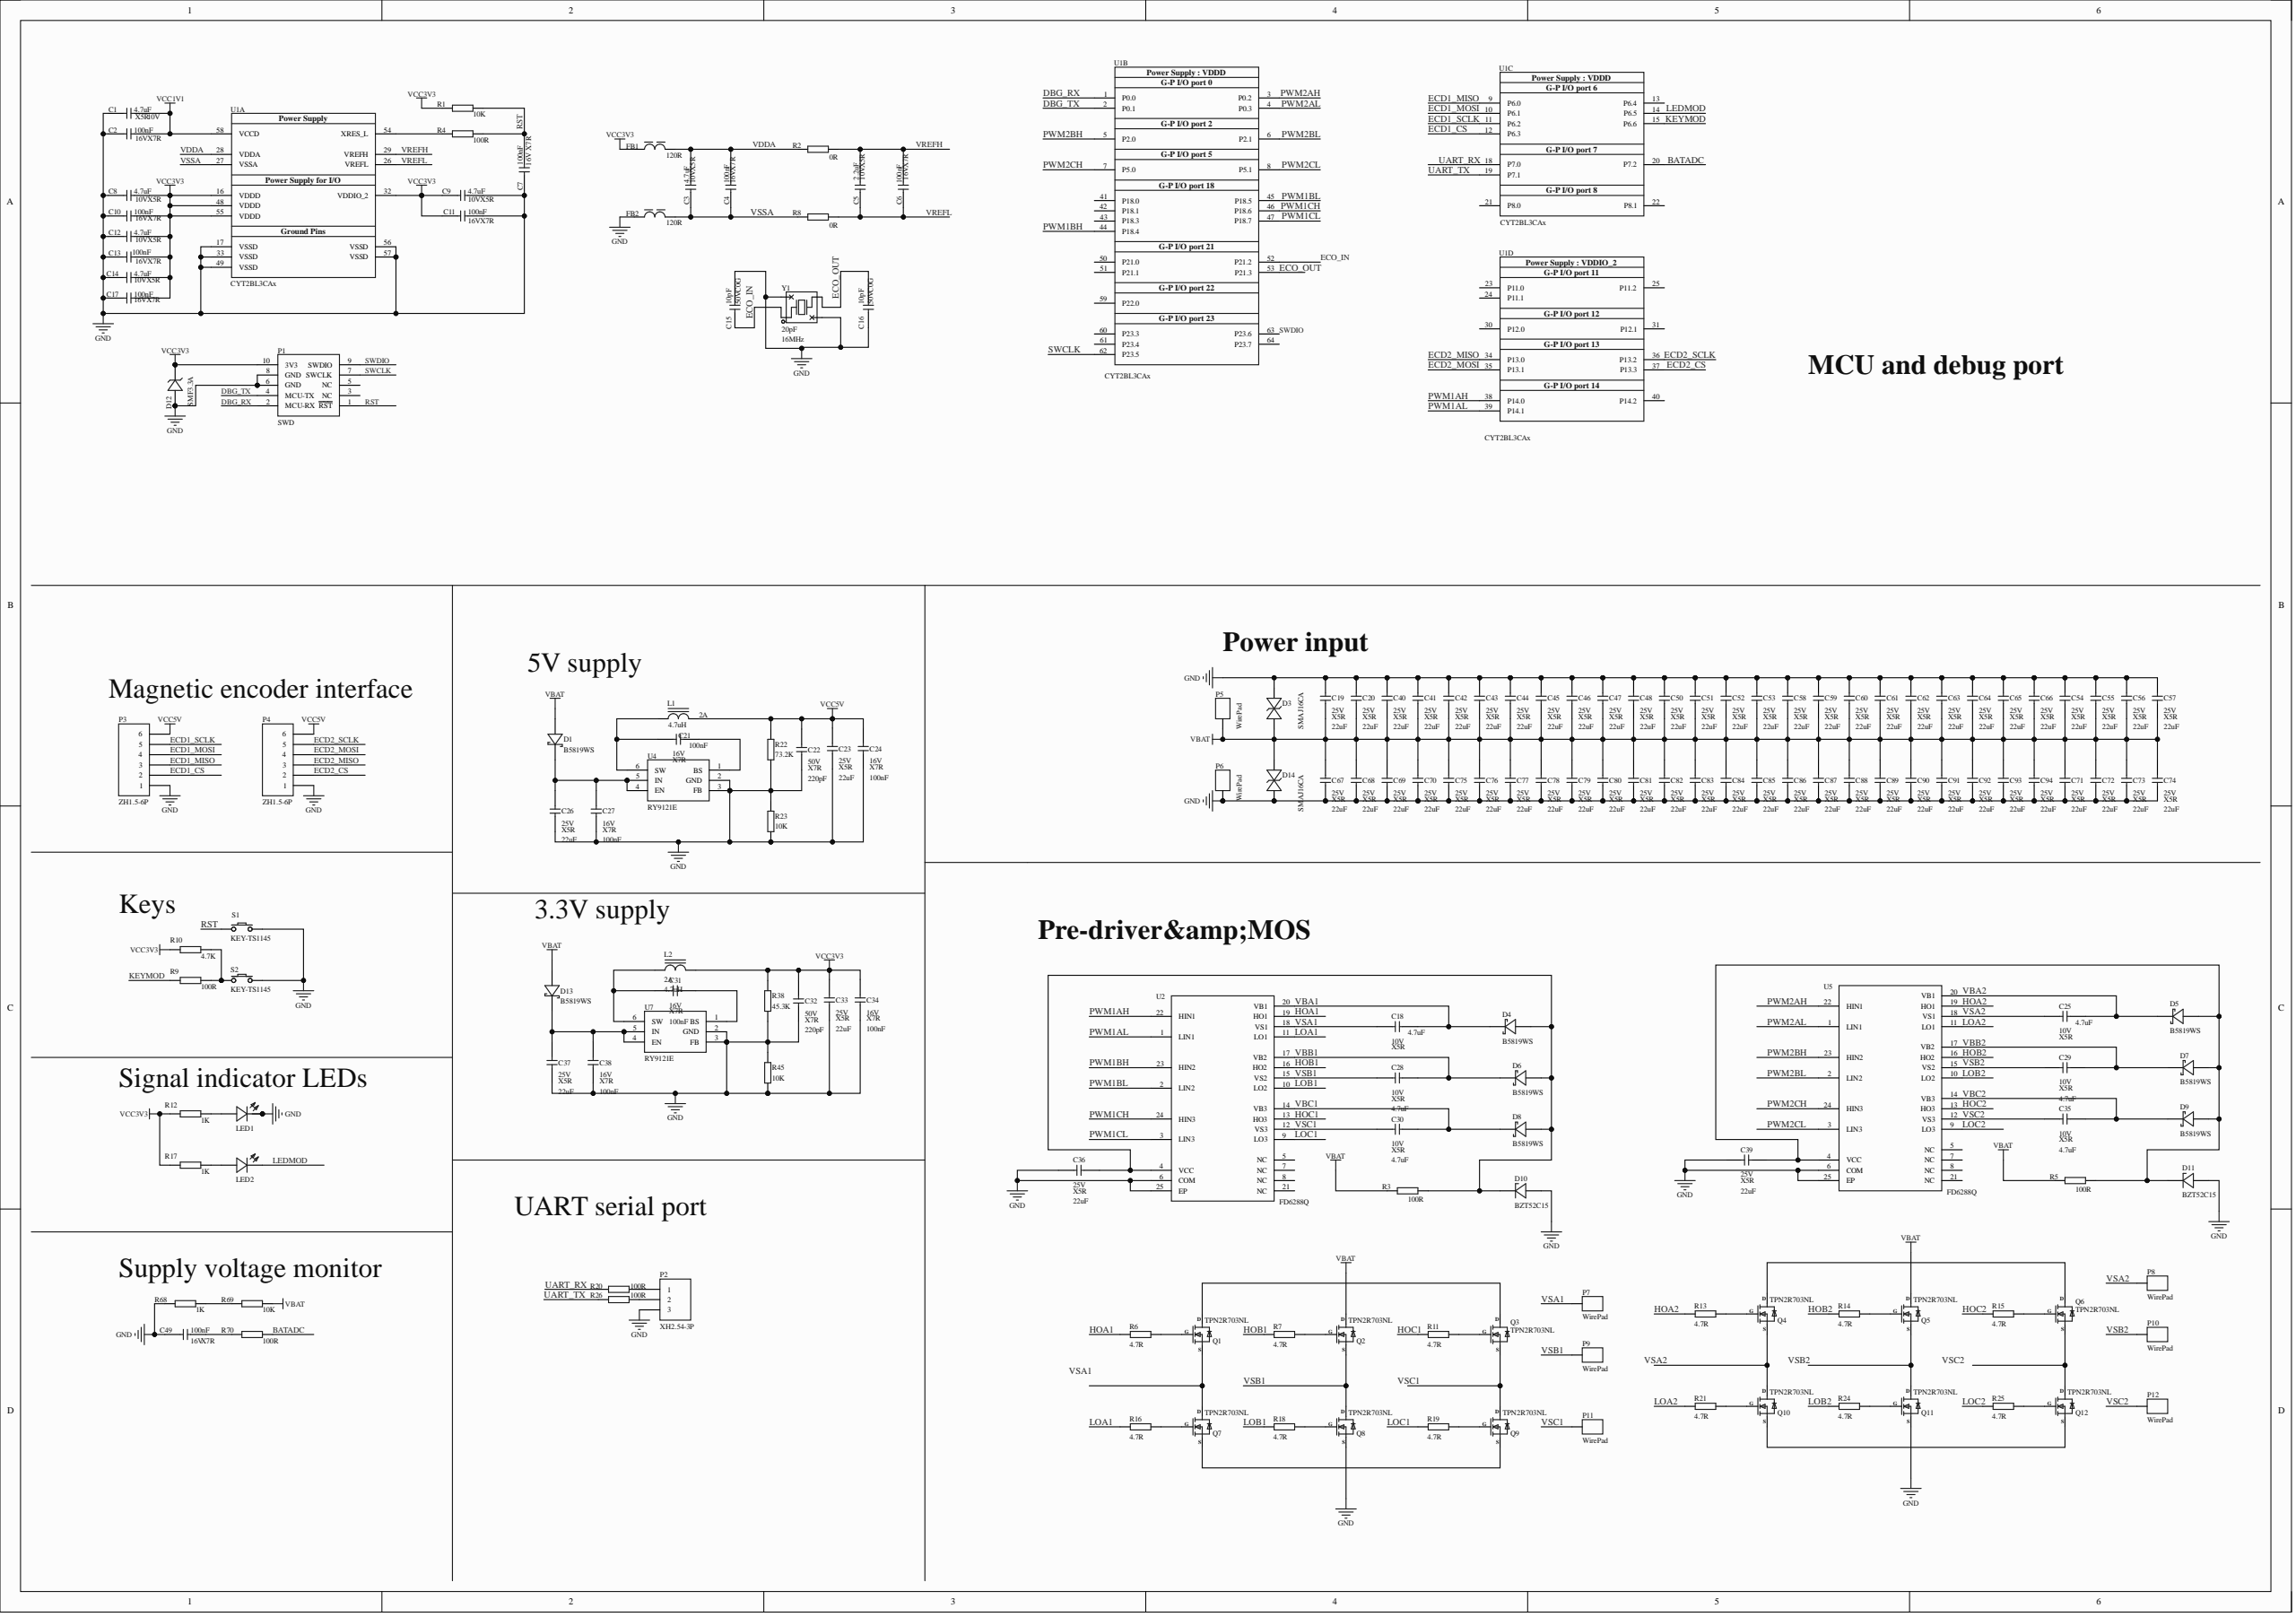Circuit board | Altium Designer | 176 parts | 102 nets
Bill of materials:
Comment,Description,Designator,Footprint,LibRef,Quantity
"","SMD ceramic capacitor; MLCC; 0402(1005);","C1, C2, C3, C4, C5, C6, C7, C8, C9, C10, C11, C12, C13, C14, C15, C16, C17, C18, C21, C22, C24, C25, C27, C28, C29, C30, C31, C32, C34, C35, C38, C49","CAPC1005[0402]S-N","=Value +' '+ Voltage + ' ' + Type","32"
"","SMD ceramic capacitor; MLCC; 0805(2012);","C19, C20, C23, C26, C33, C36, C37, C39, C40, C41, C42, C43, C44, C45, C46, C47, C48, C50, C51, C52, C53, C54, C55, C56, C57, C58, C59, C60, C61, C62, C63, C64, C65, C66, C67, C68, C69, C70, C71, C72, C73, C74, C75, C76, C77, C78, C79, C80, C81, C82, C83, C84, C85, C86, C87, C88, C89, C90, C91, C92, C93, C94","CAPC2012[0805]S-N","=Value +' '+ Voltage + ' ' + Type","62"
"B5819WS","B5819WS Schottky diode","D1, D4, D5, D6, D7, D8, D9, D13","SOD-323","B5819WS","8"
"SMAJ16CA","TRANSIENT VOLTAGE  SUPPRESSOR DIODE","D3, D14","SMA[DO-214AC]-Bi","SMAJ16CA","2"
"BZT52C15","Zener diode (voltage regulator)","D10, D11","SOD-123-L","BZT52C15","2"
"SMF3.3A","TRANSIENT VOLTAGE  SUPPRESSOR DIODE","D12","SOD-123-FL","SMF3.3A","1"
"","SMD ferrite bead","FB1, FB2","INDC1005[0402]S","=Value + ' ' + Frequency +' '+ Imax","2"
"","Power inductor","L1, L2","SLO2520","=Value + ' ' + Imax","2"
"Red SMD LED","Red SMD LED","LED1","LEDC1608(0603)-L","红色贴片LED","1"
"Blue SMD LED","Blue SMD LED","LED2","LEDC1608(0603)-L","蓝色贴片LED","1"
"SWD Header 5x2","SWD debug interface 2x5pin dual-row pin header","P1","HDR2X5-OB","SWD Header 5x2","1"
"XH2.54-3P","XH2.54-3P","P2","XH2.54-3P-SH","XH2.54-3P","1"
"ZH1.5-6P","ZH1.5-6P","P3, P4","ZH1.5-6P-SH","ZH1.5-6P","2"
"WirePad","Cable wire pad","P5, P6, P7, P8, P9, P10, P11, P12","WirePad-4x6","WirePad","8"
"TPN2R703NL","Toshiba N-channel MOS","Q1, Q2, Q3, Q4, Q5, Q6, Q7, Q8, Q9, Q10, Q11, Q12","TSON3x3","TPN2R703NL","12"
"","SMD resistor","R1, R2, R3, R4, R5, R6, R7, R8, R9, R10, R11, R12, R13, R14, R15, R16, R17, R18, R19, R20, R21, R22, R23, R24, R25, R26, R38, R45, R68, R69, R70","RESC1005[0402]S-N","=Value+' '+Tolerance","31"
"KEY-TS1145","3x4x2.5 4-pin key SMD vertical press","S1, S2","TS1145-B-A","KEY-TS1145","2"
"CYT2BL3CAx","CYT2BL3CAx","U1","LQFP64_L","CYT2BL3CAx","1"
"FD6288Q","FD6288Q three-phase gate driver","U2, U5","QFN24-4x4-L","FD6288Q","2"
"RY9121E","17V 2A 1.2MHz Synchronous Step-Down Regulator","U4, U7","SOT-23-6","RY9121E","2"
"","Four-pin passive crystal oscillator Crystal Oscillator","Y1","X3225-4","=Frequency+' '+Load_Capactiance","1"
Netlist (Protel format):
[
C1
CAPC1005[0402]S-N




]
[
C2
CAPC1005[0402]S-N




]
[
C3
CAPC1005[0402]S-N




]
[
C4
CAPC1005[0402]S-N




]
[
C5
CAPC1005[0402]S-N




]
[
C6
CAPC1005[0402]S-N




]
[
C7
CAPC1005[0402]S-N




]
[
C8
CAPC1005[0402]S-N




]
[
C9
CAPC1005[0402]S-N




]
[
C10
CAPC1005[0402]S-N




]
[
C11
CAPC1005[0402]S-N




]
[
C12
CAPC1005[0402]S-N




]
[
C13
CAPC1005[0402]S-N




]
[
C14
CAPC1005[0402]S-N




]
[
C15
CAPC1005[0402]S-N




]
[
C16
CAPC1005[0402]S-N




]
[
C17
CAPC1005[0402]S-N




]
[
C18
CAPC1005[0402]S-N




]
[
C19
CAPC2012[0805]S-N




]
[
C20
CAPC2012[0805]S-N




]
[
C21
CAPC1005[0402]S-N




]
[
C22
CAPC1005[0402]S-N




]
[
C23
CAPC2012[0805]S-N




]
[
C24
CAPC1005[0402]S-N




]
[
C25
CAPC1005[0402]S-N




]
[
C26
CAPC2012[0805]S-N




]
[
C27
CAPC1005[0402]S-N




]
[
C28
CAPC1005[0402]S-N




]
[
C29
CAPC1005[0402]S-N




]
[
C30
CAPC1005[0402]S-N




]
[
C31
CAPC1005[0402]S-N




]
[
C32
CAPC1005[0402]S-N




]
[
C33
CAPC2012[0805]S-N




]
[
C34
CAPC1005[0402]S-N




]
[
C35
CAPC1005[0402]S-N




]
[
C36
CAPC2012[0805]S-N




]
[
C37
CAPC2012[0805]S-N




]
[
C38
CAPC1005[0402]S-N




]
[
C39
CAPC2012[0805]S-N




]
[
C40
CAPC2012[0805]S-N




]
[
C41
CAPC2012[0805]S-N




]
[
C42
CAPC2012[0805]S-N




]
[
C43
CAPC2012[0805]S-N




]
[
C44
CAPC2012[0805]S-N




]
[
C45
CAPC2012[0805]S-N




]
[
C46
CAPC2012[0805]S-N




]
[
C47
CAPC2012[0805]S-N




]
[
C48
CAPC2012[0805]S-N




]
[
C49
CAPC1005[0402]S-N




]
[
C50
CAPC2012[0805]S-N




]
[
C51
CAPC2012[0805]S-N




]
[
C52
CAPC2012[0805]S-N




]
[
C53
CAPC2012[0805]S-N




]
[
C54
CAPC2012[0805]S-N




]
[
C55
CAPC2012[0805]S-N




]
[
C56
CAPC2012[0805]S-N




]
[
C57
CAPC2012[0805]S-N




]
[
C58
CAPC2012[0805]S-N




]
[
C59
CAPC2012[0805]S-N




]
[
C60
CAPC2012[0805]S-N




]
[
C61
CAPC2012[0805]S-N




]
[
C62
CAPC2012[0805]S-N




]
[
C63
CAPC2012[0805]S-N




]
[
C64
CAPC2012[0805]S-N




]
[
C65
CAPC2012[0805]S-N




]
[
C66
CAPC2012[0805]S-N




]
[
C67
CAPC2012[0805]S-N




]
[
C68
CAPC2012[0805]S-N




]
[
C69
CAPC2012[0805]S-N




]
[
C70
CAPC2012[0805]S-N




]
[
C71
CAPC2012[0805]S-N




]
[
C72
CAPC2012[0805]S-N




]
[
C73
CAPC2012[0805]S-N




]
[
C74
CAPC2012[0805]S-N




]
[
C75
CAPC2012[0805]S-N




]
[
C76
CAPC2012[0805]S-N




]
[
C77
CAPC2012[0805]S-N




]
[
C78
CAPC2012[0805]S-N




]
[
C79
CAPC2012[0805]S-N




]
[
C80
CAPC2012[0805]S-N




]
[
C81
CAPC2012[0805]S-N




]
[
C82
CAPC2012[0805]S-N




]
[
C83
CAPC2012[0805]S-N




]
[
C84
CAPC2012[0805]S-N




]
[
C85
CAPC2012[0805]S-N




]
[
C86
CAPC2012[0805]S-N




]
[
C87
CAPC2012[0805]S-N




]
[
C88
CAPC2012[0805]S-N




]
[
C89
CAPC2012[0805]S-N




]
[
C90
CAPC2012[0805]S-N




]
[
C91
CAPC2012[0805]S-N




]
[
C92
CAPC2012[0805]S-N




]
[
C93
CAPC2012[0805]S-N




]
[
C94
CAPC2012[0805]S-N




]
[
D1
SOD-323
B5819WS



]
[
D3
SMA[DO-214AC]-Bi
SMAJ16CA



]
[
D4
SOD-323
B5819WS



]
[
D5
SOD-323
B5819WS



]
[
D6
SOD-323
B5819WS



]
[
D7
SOD-323
B5819WS



]
[
D8
SOD-323
B5819WS



]
[
D9
SOD-323
B5819WS



]
[
D10
SOD-123-L
BZT52C15



]
[
D11
SOD-123-L
BZT52C15



]
[
D12
SOD-123-FL
SMF3.3A



]
[
D13
SOD-323
B5819WS



]
[
D14
SMA[DO-214AC]-Bi
SMAJ16CA



]
[
FB1
INDC1005[0402]S




]
[
FB2
INDC1005[0402]S




]
[
L1
SLO2520




]
[
L2
SLO2520




]
[
LED1
LEDC1608(0603)-L
Red SMD LED



]
[
LED2
LEDC1608(0603)-L
Blue SMD LED



]
[
P1
HDR2X5-OB
SWD Header 5x2



]
[
P2
XH2.54-3P-SH
XH2.54-3P



]
[
P3
ZH1.5-6P-SH
ZH1.5-6P



]
[
P4
ZH1.5-6P-SH
ZH1.5-6P



]
[
P5
WirePad-4x6
WirePad



]
[
P6
WirePad-4x6
WirePad



]
[
P7
WirePad-4x6
WirePad



]
[
P8
WirePad-4x6
WirePad



]
[
P9
WirePad-4x6
WirePad



]
[
P10
WirePad-4x6
WirePad



]
[
P11
WirePad-4x6
WirePad



]
[
P12
WirePad-4x6
WirePad



]
[
Q1
TSON3x3
TPN2R703NL



]
[
Q2
TSON3x3
TPN2R703NL



]
[
Q3
TSON3x3
TPN2R703NL



]
[
Q4
TSON3x3
TPN2R703NL



]
[
Q5
TSON3x3
TPN2R703NL



]
[
Q6
TSON3x3
TPN2R703NL



]
[
Q7
TSON3x3
TPN2R703NL



]
[
Q8
TSON3x3
TPN2R703NL



]
[
Q9
TSON3x3
TPN2R703NL



]
[
Q10
TSON3x3
TPN2R703NL



]
[
Q11
TSON3x3
TPN2R703NL



]
[
Q12
TSON3x3
TPN2R703NL



]
[
R1
RESC1005[0402]S-N




]
[
R2
RESC1005[0402]S-N




]
[
R3
RESC1005[0402]S-N




]
[
R4
RESC1005[0402]S-N




]
[
R5
RESC1005[0402]S-N




]
[
R6
RESC1005[0402]S-N




]
[
R7
RESC1005[0402]S-N




]
[
R8
RESC1005[0402]S-N




]
[
R9
RESC1005[0402]S-N




]
[
R10
RESC1005[0402]S-N




]
[
R11
RESC1005[0402]S-N




]
[
R12
RESC1005[0402]S-N




]
[
R13
RESC1005[0402]S-N




]
[
R14
RESC1005[0402]S-N




]
[
R15
RESC1005[0402]S-N




]
[
R16
RESC1005[0402]S-N




]
[
R17
RESC1005[0402]S-N




]
[
R18
RESC1005[0402]S-N




]
[
R19
RESC1005[0402]S-N




]
[
R20
RESC1005[0402]S-N




]
[
R21
RESC1005[0402]S-N




]
[
R22
RESC1005[0402]S-N




]
[
R23
RESC1005[0402]S-N




]
[
R24
RESC1005[0402]S-N




]
[
R25
RESC1005[0402]S-N




]
[
R26
RESC1005[0402]S-N




]
[
R38
RESC1005[0402]S-N




]
[
R45
RESC1005[0402]S-N




]
[
R68
RESC1005[0402]S-N




]
[
R69
RESC1005[0402]S-N




]
[
R70
RESC1005[0402]S-N




]
[
S1
TS1145-B-A
KEY-TS1145



]
[
S2
TS1145-B-A
KEY-TS1145



]
[
U1
LQFP64_L
CYT2BL3CAx



]
[
U2
QFN24-4x4-L
FD6288Q



]
[
U4
SOT-23-6
RY9121E



]
[
U5
QFN24-4x4-L
FD6288Q



]
[
U7
SOT-23-6
RY9121E



]
[
Y1
X3225-4




]
(
VSSA
C3-2
C4-1
FB2-2
R8-1
U1-27
)
(
VSC2
C35-1
P12-1
U5-12
)
(
VSC1
C30-1
P11-1
U2-12
)
(
VSB2
C29-1
P10-1
U5-15
)
(
VSB1
C28-1
P9-1
Q2-3
Q8-1
U2-15
)
(
VSA2
C25-1
P8-1
U5-18
)
(
VSA1
C18-1
P7-1
U2-18
)
(
VREFL
C5-1
C6-1
R8-2
U1-26
)
(
VREFH
C5-2
C6-2
R2-2
U1-29
)
(
VDDA
C3-1
C4-2
FB1-2
R2-1
U1-28
)
(
VCC5V
C22-2
C23-2
C24-2
L1-1
P3-6
P4-6
R22-2
)
(
VCC3V3
C8-2
C9-1
C10-2
C11-1
C12-2
C13-2
C14-2
C17-2
C32-2
C33-2
C34-2
D12-K
FB1-1
L2-1
P1-10
R1-1
R10-1
R12-1
R17-1
R38-2
U1-16
U1-32
U1-48
U1-55
)
(
VCC1V1
C1-2
C2-2
U1-58
)
(
VBC2
C35-2
D9-K
U5-14
)
(
VBC1
C30-2
D8-K
U2-14
)
(
VBB2
C29-2
D7-K
U5-17
)
(
VBB1
C28-2
D6-K
U2-17
)
(
VBAT
C19-1
C20-1
C40-1
C41-1
C42-1
C43-1
C44-1
C45-1
C46-1
C47-1
C48-1
C50-1
C51-1
C52-1
C53-1
C54-1
C55-1
C56-1
C57-1
C58-1
C59-1
C60-1
C61-1
C62-1
C63-1
C64-1
C65-1
C66-1
C67-2
C68-2
C69-2
C70-2
C71-2
C72-2
C73-2
C74-2
C75-2
C76-2
C77-2
C78-2
C79-2
C80-2
C81-2
C82-2
C83-2
C84-2
C85-2
C86-2
C87-2
C88-2
C89-2
C90-2
C91-2
C92-2
C93-2
C94-2
D1-A
D3-A
D13-A
D14-K
P5-1
Q2-1
Q5-1
R3-1
R5-1
R69-2
)
(
VBA2
C25-2
D5-K
U5-20
)
(
VBA1
C18-2
D4-K
U2-20
)
(
UART_TX
R26-1
U1-19
)
(
UART_RX
R20-1
U1-18
)
(
SWDIO
P1-9
U1-63
)
(
SWCLK
P1-7
U1-62
)
(
RST
C7-2
P1-1
R1-2
R4-2
S1-2
)
(
PWM2CL
U1-8
U5-3
)
(
PWM2CH
U1-7
U5-24
)
(
PWM2BL
U1-6
U5-2
)
(
PWM2BH
U1-5
U5-23
)
(
PWM2AL
U1-4
U5-1
)
(
PWM2AH
U1-3
U5-22
)
(
PWM1CL
U1-47
U2-3
)
(
PWM1CH
U1-46
U2-24
)
(
PWM1BL
U1-45
U2-2
)
(
PWM1BH
U1-44
U2-23
)
(
PWM1AL
U1-39
U2-1
)
(
PWM1AH
U1-38
U2-22
)
(
NetR68_2
R68-2
R69-1
)
(
NetR9_2
R9-2
R10-2
S2-2
)
(
NetR4_1
R4-1
U1-54
)
(
NetQ12_2
Q12-2
R25-2
)
(
NetQ11_2
Q11-2
R24-2
)
(
NetQ10_3
Q10-3
Q12-3
)
(
NetQ10_2
Q10-2
R21-2
)
(
NetQ9_2
Q9-2
R19-2
)
(
NetQ8_2
Q8-2
R18-2
)
(
NetQ7_3
Q7-3
Q9-3
)
(
NetQ7_2
Q7-2
R16-2
)
(
NetQ6_3
Q6-3
Q12-1
)
(
NetQ6_2
Q6-2
R15-2
)
(
NetQ5_3
Q5-3
Q11-1
)
(
NetQ5_2
Q5-2
R14-2
)
(
NetQ4_3
Q4-3
Q10-1
)
(
NetQ4_2
Q4-2
R13-2
)
(
NetQ4_1
Q4-1
Q6-1
)
(
NetQ3_3
Q3-3
Q9-1
)
(
NetQ3_2
Q3-2
R11-2
)
(
NetQ2_2
Q2-2
R7-2
)
(
NetQ1_3
Q1-3
Q7-1
)
(
NetQ1_2
Q1-2
R6-2
)
(
NetQ1_1
Q1-1
Q3-1
)
(
NetP2_2
P2-2
R26-2
)
(
NetP2_1
P2-1
R20-2
)
(
NetLED2_A
LED2-A
R17-2
)
(
NetLED1_A
LED1-A
R12-2
)
(
NetC49_2
C49-2
R70-1
)
(
NetC39_1
C39-1
D5-A
D7-A
D9-A
D11-K
R5-2
U5-4
)
(
NetC37_2
C37-2
C38-2
D13-K
U7-4
U7-5
)
(
NetC36_1
C36-1
D4-A
D6-A
D8-A
D10-K
R3-2
U2-4
)
(
NetC31_2
C31-2
L2-2
U7-6
)
(
NetC31_1
C31-1
U7-1
)
(
NetC26_2
C26-2
C27-2
D1-K
U4-4
U4-5
)
(
NetC21_2
C21-2
L1-2
U4-6
)
(
NetC21_1
C21-1
U4-1
)
(
LOC2
R25-1
U5-9
)
(
LOC1
R19-1
U2-9
)
(
LOB2
R24-1
U5-10
)
(
LOB1
R18-1
U2-10
)
(
LOA2
R21-1
U5-11
)
(
LOA1
R16-1
U2-11
)
(
LEDMOD
LED2-C
U1-14
)
(
KEYMOD
R9-1
U1-15
)
(
HOC2
R15-1
U5-13
)
(
HOC1
R11-1
U2-13
)
(
HOB2
R14-1
U5-16
)
(
HOB1
R7-1
U2-16
)
(
HOA2
R13-1
U5-19
)
(
HOA1
R6-1
U2-19
)
(
GND
C1-1
C2-1
C7-1
C8-1
C9-2
C10-1
C11-2
C12-1
C13-1
C14-1
C15-2
C16-1
C17-1
C19-2
C20-2
C22-1
C23-1
C24-1
C26-1
C27-1
C32-1
C33-1
C34-1
C36-2
C37-1
C38-1
C39-2
C40-2
C41-2
C42-2
C43-2
C44-2
C45-2
C46-2
C47-2
C48-2
C49-1
C50-2
C51-2
C52-2
C53-2
C54-2
C55-2
C56-2
C57-2
C58-2
C59-2
C60-2
C61-2
C62-2
C63-2
C64-2
C65-2
C66-2
C67-1
C68-1
C69-1
C70-1
C71-1
C72-1
C73-1
C74-1
C75-1
C76-1
C77-1
C78-1
C79-1
C80-1
C81-1
C82-1
C83-1
C84-1
C85-1
C86-1
C87-1
C88-1
C89-1
C90-1
C91-1
C92-1
C93-1
C94-1
D3-K
D10-A
D11-A
D12-A
D14-A
FB2-1
LED1-C
P1-6
P1-8
P2-3
P3-1
P4-1
P6-1
Q8-3
Q11-3
R22-1
R23-1
R23-2
R38-1
R45-1
R45-2
R68-1
S1-1
S2-1
U1-17
U1-33
U1-49
U1-56
U1-57
U2-6
U2-25
U4-2
U4-3
U5-6
U5-25
U7-2
U7-3
Y1-2
Y1-4
)
(
ECO_OUT
C16-2
U1-53
Y1-3
)
(
ECO_IN
C15-1
U1-52
Y1-1
)
(
ECD2_SCLK
P4-5
U1-36
)
(
ECD2_MOSI
P4-4
U1-35
)
(
ECD2_MISO
P4-3
U1-34
)
(
ECD2_CS
P4-2
U1-37
)
(
ECD1_SCLK
P3-5
U1-11
)
(
ECD1_MOSI
P3-4
U1-10
)
(
ECD1_MISO
P3-3
U1-9
)
(
ECD1_CS
P3-2
U1-12
)
(
DBG_TX
P1-4
U1-2
)
(
DBG_RX
P1-2
U1-1
)
(
BATADC
R70-2
U1-20
)